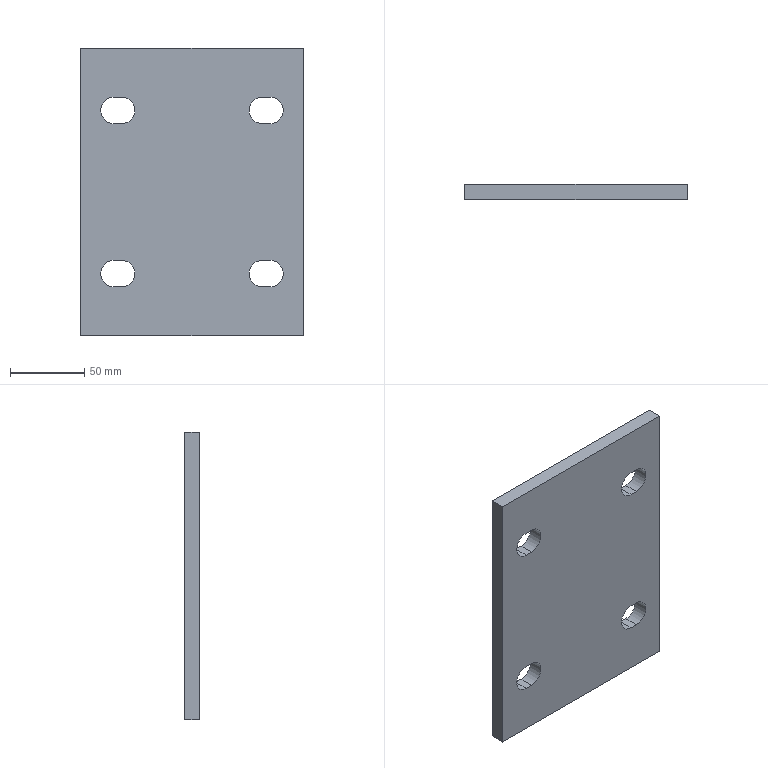Part | STEP file | Column lower connecting plate 200×150 | 1 solid | 22 faces | box 150 x 10 x 194 mm | volume 277221 mm3 | plane 14 | cylinder 8 | commonest cylinder face diameters 18 x8